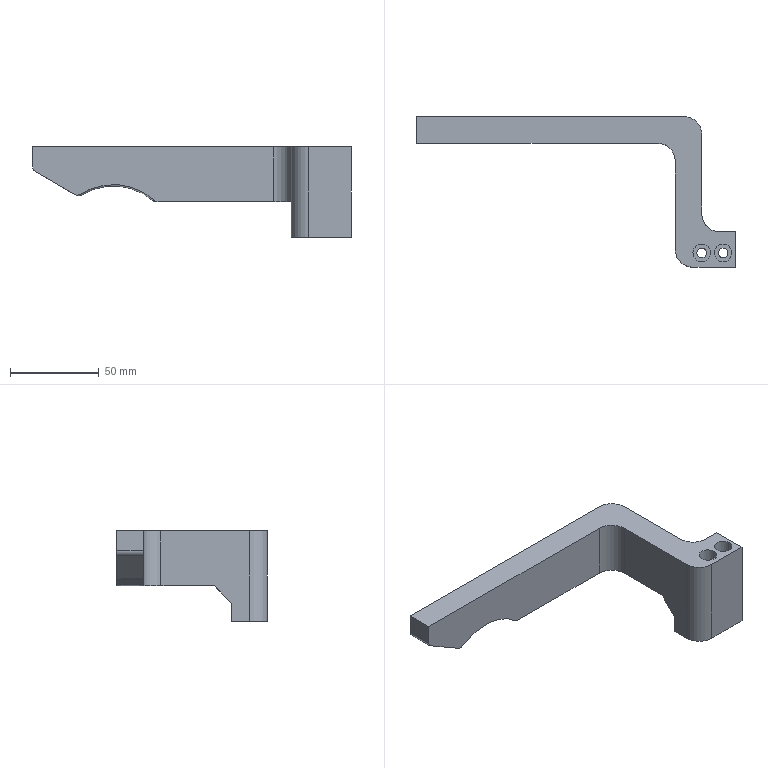NC program | NX | posted with a generic post | part box 180 x 85 x 51 mm
Lines 24 to 1125 of 44959:
(ADAPTIVE_MILLING , TOOL : D12C)
N46 T12 M6
N48 G54
N50 G17 G0 G90 X104.183 Y22.541 S9500 M3
N52 G43 Z30. H12
N54 Z-23.
N56 G94 G1 Z-26. F1000.
N58 X102.633 Y23.218 F3000.
N60 G3 X101.017 Y22.541 R1.217
N62 X100.588 Y19.038 R13.703
N64 X100.502 Y0.139 R864.64
N66 G1 X100.501 Y-45.049
N68 X100.5 Y-45.199
N70 X100.497 Y-45.311
N72 X100.491 Y-45.424
N74 X100.483 Y-45.536
N76 G2 X96.9 Y-50.921 R7.15
N78 X90.805 Y-52.726 R14.272
N80 X81.774 Y-52.986 R105.312
N82 G1 X79.862 Y-52.99
N84 X76.637 Y-52.992
N86 X64.712
N88 X-92.638 Y-52.991
N90 X-92.713 Y-52.99
N92 X-92.826 Y-52.986
N94 G2 X-98.231 Y-49.705 R6.988
N96 X-100.165 Y-43.85 R13.204
N98 X-100.483 Y-34.823 R85.978
N100 G1 X-100.487 Y-33.135
N102 X-100.49 Y-30.548
N104 X-100.491 Y-24.585
N106 Y45.127
N108 X-100.489 Y45.24
N110 X-100.485 Y45.352
N112 G2 X-97.049 Y50.824 R7.048
N114 X-90.979 Y52.706 R13.869
N116 X-81.425 Y52.986 R104.172
N118 G1 X-79.362 Y52.989
N120 X-75.575 Y52.991
N122 X-41.112
N124 X92.65
N126 X92.763 Y52.989
N128 X92.875 Y52.984
N130 G2 X98.336 Y49.53 R7.063
N132 X100.198 Y43.532 R13.787
N134 X100.485 Y34.128 R99.972
N136 X100.443 Y24.191 R284.848
N138 G3 X100.015 Y11.078 R148.084
N140 G1 X100.011 Y8.978
N142 X100.009 Y5.453
N144 X100.008 Y-5.872
N146 X100.007 Y-42.622
N148 Y-42.735
N150 X100.004 Y-42.885
N152 G2 X95.318 Y-50.333 R8.732
N154 X88.759 Y-52.177 R16.71
N156 X79.355 Y-52.477 R105.888
N158 G1 X77.705 Y-52.481
N160 X75.305 Y-52.485
N162 X70.73 Y-52.486
N164 X-31.645
N166 X-33.895 Y-52.49
N168 X-36.108 Y-52.491
N170 X-38.358 Y-52.489
N172 X-40.683 Y-52.491
N174 X-42.858 Y-52.489
N176 X-45.183 Y-52.491
N178 X-47.47 Y-52.489
N180 X-50.245 Y-52.49
N182 X-52.458 Y-52.489
N184 X-54.783 Y-52.49
N186 X-57.07 Y-52.489
N188 X-59.845 Y-52.49
N190 X-62.02 Y-52.489
N192 X-64.345 Y-52.49
N194 X-66.633 Y-52.489
N196 X-69.295 Y-52.49
N198 X-71.583 Y-52.489
N200 X-73.908 Y-52.49
N202 X-76.195 Y-52.489
N204 X-78.97 Y-52.49
N206 X-81.183 Y-52.489
N208 X-83.508 Y-52.49
N210 X-85.795 Y-52.489
N212 X-88.57 Y-52.49
N214 X-90.258 Y-52.489
N216 X-90.408 Y-52.487
N218 X-90.558 Y-52.482
N220 X-90.708 Y-52.476
N222 X-90.82 Y-52.469
N224 G2 X-97.829 Y-47.823 R8.734
N226 X-99.685 Y-41.19 R16.83
N228 X-99.979 Y-30.96 R119.013
N230 G1 X-99.982 Y-28.973
N232 X-99.985 Y-25.673
N234 X-99.986 Y-15.585
N236 X-99.985 Y42.765
N238 X-99.983 Y42.915
N240 X-99.978 Y43.064
N242 G2 X-95.308 Y50.33 R8.727
N244 X-88.749 Y52.175 R16.689
N246 X-77.995 Y52.48 R120.763
N248 G1 X-75.745 Y52.483
N250 X-71.77 Y52.485
N252 X-43.458 Y52.486
N254 X90.267 Y52.485
N256 X90.38 Y52.483
N258 X90.492 Y52.481
N260 G2 X97.756 Y47.936 R8.688
N262 X99.651 Y41.47 R16.28
N264 X99.977 Y31.467 R104.384
N266 X99.663 Y19.737 R156.739
N268 G3 X99.514 Y0.726 R633.906
N270 G1 X99.513 Y-40.261
N272 X99.512 Y-40.524
N274 X99.51 Y-40.749
N276 X99.507 Y-40.974
N278 X99.5 Y-41.198
N280 X99.492 Y-41.386
N282 G2 X93.807 Y-49.9 R9.898
N284 X86.723 Y-51.686 R19.459
N286 X75.967 Y-51.974 R137.207
N288 G1 X73.867 Y-51.978
N290 X70.492 Y-51.98
N292 X61.23 Y-51.981
N294 X-29.22 Y-51.98
N296 X-31.545 Y-51.985
N298 X-33.833 Y-51.986
N300 X-35.97
N302 X-38.295 Y-51.988
N304 X-40.583
N306 X-41.558 Y-51.987
N308 X-43.883 Y-51.989
N310 X-46.17 Y-51.988
N312 X-46.508
N314 X-48.758 Y-51.989
N316 X-50.82 Y-51.987
N318 X-53.07 Y-51.988
N320 X-55.133 Y-51.987
N322 X-57.458 Y-51.988
N324 X-59.745 Y-51.987
N326 X-62.258 Y-51.988
N328 X-64.583 Y-51.987
N330 X-66.833 Y-51.988
N332 X-68.745 Y-51.986
N334 X-70.995 Y-51.988
N336 X-72.908 Y-51.987
N338 X-75.158 Y-51.988
N340 X-77.258 Y-51.987
N342 X-79.508 Y-51.989
N344 X-81.608 Y-51.987
N346 X-83.858 Y-51.989
N348 X-85.958 Y-51.988
N350 G2 X-90.261 Y-51.823 R26.749
N352 X-97.485 Y-46.13 R9.964
N354 X-99.186 Y-39.213 R19.73
N356 X-99.473 Y-28.383 R138.479
N358 G1 X-99.477 Y-26.283
N360 X-99.479 Y-22.87
N362 X-99.48 Y-13.083
N364 Y40.617
N366 X-99.478 Y40.805
N368 X-99.476 Y40.955
N370 G2 X-93.801 Y49.893 R9.889
N372 X-86.83 Y51.673 R19.285
N374 X-76.375 Y51.971 R128.078
N376 G1 X-74.463 Y51.975
N378 X-71.575 Y51.978
N380 X-65.35 Y51.98
N382 X88.1 Y51.979
N384 X88.287 Y51.978
N386 X88.512 Y51.975
N388 G2 X97.385 Y46.316 R9.878
N390 X99.185 Y39.198 R19.477
N392 X99.224 Y21.172 R144.828
N394 G3 X99.013 Y0.362 R556.134
N396 G1 X99.011 Y-1.551
N398 X99.012 Y-3.801
N400 X99.011 Y-5.638
N402 X99.013 Y-7.963
N404 X99.011 Y-10.251
N406 X99.012 Y-11.376
N408 Y-13.663
N410 X99.011 Y-15.276
N412 X99.012 Y-17.601
N414 X99.011 Y-19.888
N416 X99.012 Y-22.438
N418 X99.011 Y-24.238
N420 X99.012 Y-26.563
N422 X99.011 Y-28.851
N424 Y-29.113
N426 X99.012 Y-31.363
N428 X99.01 Y-33.313
N430 G2 X98.946 Y-40.436 R135.893
N432 X92.544 Y-49.421 R10.75
N434 X85.327 Y-51.161 R21.244
N436 X74.46 Y-51.466 R137.759
N438 G1 X72.622 Y-51.47
N440 X69.885 Y-51.473
N442 X64.597 Y-51.475
N444 X4.11
N446 X1.86 Y-51.479
N448 X-0.353 Y-51.48
N450 X-2.603 Y-51.478
N452 X-4.853 Y-51.479
N454 X-6.615 Y-51.478
N456 X-8.865 Y-51.479
N458 X-10.89 Y-51.478
N460 X-13.14 Y-51.479
N462 X-15.165 Y-51.478
N464 X-17.415 Y-51.479
N466 X-19.403 Y-51.478
N468 X-21.653 Y-51.479
N470 X-23.678 Y-51.478
N472 X-25.928 Y-51.479
N474 X-27.39 Y-51.478
N476 X-29.715 Y-51.481
N478 X-30.765
N480 X-33.015 Y-51.485
N482 X-35.228 Y-51.486
N484 X-36.39 Y-51.485
N486 X-38.64 Y-51.487
N488 X-40.853 Y-51.486
N490 X-43.59 Y-51.488
N492 X-45.578 Y-51.486
N494 X-47.828 Y-51.487
N496 X-49.89 Y-51.486
N498 X-52.215 Y-51.487
N500 X-54.503 Y-51.486
N502 X-57.053 Y-51.487
N504 X-58.928 Y-51.486
N506 X-61.253 Y-51.487
N508 X-63.54 Y-51.486
N510 X-66.278
N512 X-67.853 Y-51.485
N514 X-70.103 Y-51.486
N516 X-71.94 Y-51.485
N518 X-74.19 Y-51.487
N520 X-76.253 Y-51.486
N522 X-78.503 Y-51.487
N524 X-80.565 Y-51.486
N526 X-82.815 Y-51.487
N528 X-84.878 Y-51.486
N530 G2 X-89.654 Y-51.157 R20.334
N532 X-96.946 Y-44.982 R10.805
N534 X-98.662 Y-37.797 R21.426
N536 X-98.964 Y-27.042 R137.503
N538 G1 X-98.969 Y-25.167
N540 X-98.972 Y-22.429
N542 X-98.974 Y-17.217
N544 Y38.771
N546 X-98.972 Y39.071
N548 X-98.97 Y39.258
N550 G2 X-92.432 Y49.462 R10.813
N552 X-84.945 Y51.195 R22.037
N554 X-72.838 Y51.469 R170.072
N556 G1 X-70.176 Y51.472
N558 X-65.226 Y51.474
N560 X86.274
N562 X86.574 Y51.472
N564 X86.762 Y51.469
N566 X86.949 Y51.466
N568 G2 X96.9 Y45.064 R10.771
N570 X98.663 Y37.777 R21.258
N572 X98.79 Y23.012 R121.633
N574 G3 X98.51 Y0.365 R561.198
N576 G1 X98.511 Y-1.96
N578 X98.509 Y-3.835
N580 X98.511 Y-6.16
N582 X98.509 Y-8.448
N584 X98.511 Y-10.96
N586 X98.509 Y-13.21
N588 X98.51 Y-15.722
N590 X98.509 Y-18.01
N592 X98.51 Y-20.41
N594 X98.509 Y-22.735
N596 X98.511 Y-25.06
N598 X98.509 Y-27.347
N600 Y-27.647
N602 X98.51 Y-29.972
N604 X98.509 Y-32.297
N606 X98.511 Y-34.622
N608 G2 X98.321 Y-40.126 R39.885
N610 X91.512 Y-48.883 R11.401
N612 X84.141 Y-50.633 R22.526
N614 X73.162 Y-50.958 R136.895
N616 G1 X71.399 Y-50.963
N618 X68.924 Y-50.967
N620 X64.799 Y-50.969
N622 X49.499
N624 X6.524
N626 X4.199 Y-50.974
N628 X1.912 Y-50.975
N630 X-0.263 Y-50.974
N632 X-2.588 Y-50.977
N634 X-4.876
N636 X-5.888 Y-50.976
N638 X-8.213 Y-50.978
N640 X-10.501 Y-50.977
N642 X-10.838
N644 X-13.163 Y-50.978
N646 X-15.451 Y-50.977
N648 X-18.188
N650 X-19.763 Y-50.976
N652 X-22.088 Y-50.978
N654 X-24.376 Y-50.977
N656 X-24.901 Y-50.976
N658 X-27.151 Y-50.977
N660 X-27.863
N662 X-30.113 Y-50.979
N664 X-31.126 Y-50.98
N666 X-33.376 Y-50.984
N668 X-35.588 Y-50.985
N670 X-37.051 Y-50.984
N672 X-39.301 Y-50.986
N674 X-41.513 Y-50.985
N676 X-44.176 Y-50.987
N678 X-46.463 Y-50.985
N680 X-47.176 Y-50.984
N682 X-49.426 Y-50.985
N684 X-50.701 Y-50.984
N686 X-52.951 Y-50.986
N688 X-55.163 Y-50.985
N690 X-55.538 Y-50.984
N692 X-57.788 Y-50.985
N694 X-59.401 Y-50.984
N696 X-61.726 Y-50.986
N698 X-64.013 Y-50.985
N700 X-64.876 Y-50.984
N702 X-67.126
N704 X-68.476 Y-50.983
N706 X-70.726 Y-50.985
N708 X-72.751 Y-50.984
N710 X-75.001 Y-50.985
N712 G2 X-86.437 Y-50.929 R334.978
N714 X-96.37 Y-44.025 R11.416
N716 X-98.16 Y-36.32 R22.954
N718 X-98.461 Y-24.177 R164.437
N720 G1 X-98.465 Y-21.852
N722 X-98.468 Y-18.102
N724 X-98.469 Y-7.415
N726 X-98.468 Y37.135
N728 Y37.285
N730 X-98.465 Y37.623
N732 G2 X-96.76 Y44.366 R12.529
N734 X-89.843 Y49.53 R12.587
N736 X-81.717 Y50.8 R30.53
N738 X-64.395 Y50.968 R454.906
N740 G1 X-44.407
N742 X84.63
N744 X84.78 Y50.967
N746 X85.118 Y50.964
N748 X85.38 Y50.96
N750 X85.68 Y50.952
N752 G2 X94.217 Y47.301 R11.485
N754 X97.644 Y40.029 R15.153
N756 X98.396 Y31.298 R49.905
N758 X98.156 Y18.965 R259.207
N760 G3 X98.009 Y-4.322 R927.895
N762 G1 X98.007 Y-6.459
N764 X98.009 Y-8.784
N766 X98.007 Y-11.034
N768 X98.008 Y-13.547
N770 X98.007 Y-15.872
N772 X98.008 Y-18.197
N774 X98.007 Y-20.522
N776 X98.008 Y-22.847
N778 G2 X97.966 Y-37.321 R804.806
N780 X94.215 Y-45.957 R12.099
N782 X86.962 Y-49.517 R15.409
N784 X78.393 Y-50.366 R46.017
N786 X60.018 Y-50.464 R838.629
N788 G1 X8.943
N790 X6.618 Y-50.468
N792 X4.331 Y-50.47
N794 X1.893
N796 X-0.432 Y-50.474
N798 X-2.719 Y-50.475
N800 X-4.444 Y-50.474
N802 X-6.769 Y-50.476
N804 X-9.057
N806 X-9.694 Y-50.475
N808 X-12.019 Y-50.477
N810 X-14.307 Y-50.475
N812 X-14.682
N814 X-16.932 Y-50.476
N816 X-18.694 Y-50.475
N818 X-21.019 Y-50.477
N820 X-23.307 Y-50.475
N822 X-23.832
N824 X-26.157 Y-50.476
N826 X-27.432 Y-50.475
N828 X-29.757 Y-50.478
N830 X-31.032 Y-50.479
N832 X-33.282 Y-50.482
N834 X-35.494 Y-50.483
N836 X-36.657
N838 X-38.907 Y-50.484
N840 X-41.157
N842 X-43.407 Y-50.485
N844 X-45.619 Y-50.484
N846 X-46.144 Y-50.483
N848 X-48.469 Y-50.484
N850 X-50.269 Y-50.483
N852 X-52.594 Y-50.485
N854 X-54.882 Y-50.484
N856 X-55.519 Y-50.483
N858 X-57.769 Y-50.484
N860 X-59.194 Y-50.483
N862 X-61.444 Y-50.485
N864 X-63.657 Y-50.483
N866 X-64.219
N868 X-66.469
N870 G2 X-84.881 Y-50.441 R991.792
N872 X-91.413 Y-48.478 R12.976
N874 X-95.973 Y-43.934 R6.278
N876 X-97.794 Y-33.025 R38.287
N878 X-97.962 Y-15.252 R491.479
N880 G1 X-97.963 Y0.948
N882 Y35.598
N884 X-97.962 Y35.786
N886 X-97.959 Y36.123
N888 X-97.955 Y36.423
N890 X-97.95 Y36.686
N892 G2 X-95.932 Y43.912 R13.045
N894 X-88.775 Y49.02 R13.286
N896 X-80.795 Y50.269 R31.53
N898 X-63.623 Y50.462 R400.009
N900 G1 X-52.748 Y50.463
N902 X83.077 Y50.462
N904 X83.302
N906 X83.602 Y50.459
N908 X83.902 Y50.455
N910 X84.127 Y50.451
N912 G2 X91.397 Y48.481 R13.562
N914 X95.973 Y43.934 R6.277
N916 X97.776 Y33.361 R37.715
N918 X97.743 Y22.227 R138.477
N920 G3 X97.506 Y-5.183 R921.948
N922 G1 X97.507 Y-7.508
N924 X97.506 Y-9.796
N926 X97.507 Y-12.121
N928 X97.505 Y-14.446
N930 X97.507 Y-16.771
N932 X97.505 Y-19.021
N934 X97.507 Y-21.533
N936 X97.505 Y-23.821
N938 G2 X97.446 Y-36.42 R413.025
N940 X93.853 Y-44.997 R12.689
N942 X86.332 Y-48.909 R15.522
N944 X77.359 Y-49.85 R45.736
N946 X60.935 Y-49.957 R763.704
N948 G1 X45.335 Y-49.958
N950 X11.36
N952 X9.035 Y-49.962
N954 X6.747 Y-49.964
N956 X4.272
N958 X1.947 Y-49.969
N960 X-0.34 Y-49.97
N962 X-2.028
N964 X-4.353 Y-49.973
N966 X-6.64 Y-49.974
N968 X-7.878 Y-49.973
N970 X-10.203 Y-49.975
N972 X-12.49 Y-49.974
N974 X-13.053 Y-49.973
N976 X-15.378 Y-49.975
N978 X-17.665 Y-49.973
N980 X-19.99 Y-49.975
N982 X-22.278 Y-49.974
N984 X-22.803 Y-49.973
N986 X-25.128 Y-49.975
N988 X-26.628 Y-49.974
N990 X-28.878 Y-49.976
N992 X-29.965
N994 X-32.215 Y-49.98
N996 X-34.428
N998 X-34.99
N1000 X-37.24 Y-49.982
N1002 X-39.453 Y-49.981
N1004 X-42.228 Y-49.983
N1006 X-44.515 Y-49.982
N1008 X-45.04
N1010 X-47.365 Y-49.983
N1012 X-49.503 Y-49.982
N1014 X-51.828 Y-49.984
N1016 X-54.115 Y-49.982
N1018 X-54.715
N1020 X-57.04 Y-49.983
N1022 X-58.99 Y-49.982
N1024 X-61.315 Y-49.984
N1026 X-63.603 Y-49.982
N1028 X-64.578 Y-49.981
N1030 X-66.828 Y-49.982
N1032 X-68.14 Y-49.981
N1034 X-70.465 Y-49.982
N1036 X-72.753 Y-49.981
N1038 X-73.09
N1040 X-75.34 Y-49.982
N1042 X-76.878 Y-49.981
N1044 G2 X-84.525 Y-49.88 R113.76
N1046 X-89.461 Y-48.669 R19.083
N1048 X-91.434 Y-48.473 R27.743
N1050 G1 X-91.3 Y-48.504
N1052 X-89.965 Y-48.65
N1054 X-89.614
N1056 G2 X-86.891 Y-49.168 R25.774
N1058 G3 X-79.306 Y-49.667 R43.084
N1060 G1 X-78.368 Y-49.672
N1062 X-76.756 Y-49.676
N1064 X-74.918 Y-49.678
N1066 X-73.793 Y-49.679
N1068 X-73.156 Y-49.68
N1070 X-71.731
N1072 X-70.756 Y-49.681
N1074 X-69.818 Y-49.68
N1076 X-69.368
N1078 X-68.018 Y-49.681
N1080 X-67.306
N1082 X-66.818 Y-49.682
N1084 X-66.443 Y-49.681
N1086 X-65.731 Y-49.682
N1088 X-65.168
N1090 X-63.781 Y-49.683
N1092 X-62.281
N1094 X-61.718
N1096 X-60.931 Y-49.682
N1098 X-60.293
N1100 X-59.206 Y-49.683
N1102 X-58.493
N1104 X-58.043
N1106 X-56.581 Y-49.682
N1108 X-54.743 Y-49.683
N1110 X-53.431
N1112 X-52.906
N1114 X-52.456
N1116 X-50.993 Y-49.682
N1118 X-50.506 Y-49.683
N1120 X-49.831
N1122 X-49.418
N1124 X-48.518
N1126 X-46.681 Y-49.682
N1128 X-45.968 Y-49.683
N1130 X-44.693
N1132 X-44.131
N1134 X-43.043
N1136 X-42.518
N1138 X-41.393 Y-49.682
N1140 X-40.868
N1142 X-39.893 Y-49.683
N1144 X-39.556 Y-49.682
N1146 X-39.181 Y-49.683
N1148 X-38.168 Y-49.682
N1150 X-37.643
N1152 X-37.118 Y-49.681
N1154 X-36.706
N1156 X-34.943
N1158 X-34.606
N1160 X-34.268
N1162 X-33.556 Y-49.68
N1164 X-32.806
N1166 X-31.681 Y-49.678
N1168 X-31.231
N1170 X-30.331 Y-49.677
N1172 X-29.993
N1174 X-28.193 Y-49.675
N1176 X-27.706
N1178 X-26.356
N1180 X-25.793
N1182 X-24.218 Y-49.674
N1184 X-23.768
N1186 X-23.168 Y-49.675
N1188 X-22.718 Y-49.674
N1190 X-22.118
N1192 X-20.993 Y-49.675
N1194 X-20.281
N1196 X-18.931 Y-49.674
N1198 X-18.443
N1200 X-18.106
N1202 X-17.656
N1204 X-16.981 Y-49.675
N1206 X-15.931 Y-49.674
N1208 X-15.518 Y-49.675
N1210 X-14.468 Y-49.674
N1212 X-13.343 Y-49.675
N1214 X-12.856
N1216 X-11.768
N1218 X-10.343 Y-49.674
N1220 X-9.181 Y-49.673
N1222 X-8.056 Y-49.674
N1224 X-7.343
N1226 X-5.506 Y-49.673
N1228 X-3.968 Y-49.671
N1230 X-2.243
N1232 X-1.156
N1234 X-0.106 Y-49.67
N1236 X0.419 Y-49.669
N1238 X0.982
N1240 X1.732 Y-49.668
N1242 X2.632 Y-49.666
N1244 X4.919
N1246 X6.007 Y-49.665
N1248 X7.619 Y-49.663
N1250 X7.994
N1252 X8.782 Y-49.662
N1254 X9.457 Y-49.66
N1256 X10.282
N1258 X11.782 Y-49.659
N1260 X13.132
N1262 X13.469 Y-49.658
N1264 X13.882 Y-49.659
N1266 X14.482 Y-49.658
N1268 X14.932
N1270 X15.607
N1272 X16.732
N1274 X17.332
N1276 X17.969
N1278 X18.719
N1280 X19.469
N1282 X20.219
N1284 X21.082
N1286 X21.569
N1288 X22.019
N1290 X23.369
N1292 X24.494
N1294 X25.057
N1296 X25.769
N1298 X26.144
N1300 X27.119
N1302 X28.507
N1304 X30.269 Y-49.657
N1306 X30.644 Y-49.658
N1308 X31.057 Y-49.657
N1310 X32.444 Y-49.658
N1312 X32.969 Y-49.657
N1314 X33.307 Y-49.658
N1316 X33.719 Y-49.657
N1318 X35.069 Y-49.658
N1320 X35.594
N1322 X36.007
N1324 X36.344
N1326 X36.719
N1328 X37.694
N1330 X39.082
N1332 X40.844
N1334 X41.182
N1336 X41.594
N1338 X42.194 Y-49.657
N1340 X42.682 Y-49.658
N1342 X43.882 Y-49.657
N1344 X45.007
N1346 X45.569 Y-49.658
N1348 X46.432
N1350 X46.844
N1352 X47.819
N1354 X48.757
N1356 X49.732
N1358 X50.669
N1360 X51.644
N1362 X53.032
N1364 X53.632
N1366 X54.869 Y-49.657
N1368 X55.207 Y-49.658
N1370 X56.332 Y-49.657
N1372 X56.669 Y-49.658
N1374 X57.119 Y-49.657
N1376 X58.282
N1378 X58.844 Y-49.658
N1380 X59.519
N1382 X59.932 Y-49.657
N1384 X61.057
N1386 X61.582
N1388 X63.157 Y-49.656
N1390 X63.494
N1392 X64.207 Y-49.655
N1394 X65.032 Y-49.654
N1396 X65.482
N1398 G3 X80.028 Y-49.412 R272.344
N1400 X88.228 Y-47.93 R29.327
N1402 X95.619 Y-41.556 R12.873
N1404 X97.103 Y-34.791 R17.08
N1406 X97.206 Y-19.267 R485.423
N1408 G1 Y-17.28
N1410 X97.205 Y-16.005
N1412 X97.206 Y-15.217
N1414 Y-13.38
N1416 Y-12.855
N1418 Y-12.217
N1420 Y-11.092
N1422 X97.207 Y-8.805
N1424 X97.206 Y-6.967
N1426 X97.207 Y-6.217
N1428 X97.208 Y-4.68
N1430 Y-3.517
N1432 Y-2.242
N1434 G2 X97.564 Y27.679 R972.698
N1436 G3 X96.866 Y38.93 R64.756
N1438 X96.15 Y42.203 R153.829
N1440 X95.973 Y43.934 R27.64
N1442 G1 X96.004 Y43.8
N1444 X96.15 Y42.465
N1446 Y42.203
N1448 G3 X96.568 Y37.613 R40.294
N1450 G2 X96.967 Y23.642 R101.585
N1452 G3 X96.705 Y-4.968 R948.71
N1454 G1 X96.706 Y-7.293
N1456 X96.704 Y-9.393
N1458 X96.705 Y-11.718
N1460 X96.703 Y-14.005
N1462 X96.705 Y-16.518
N1464 X96.703 Y-18.805
N1466 Y-19.068
N1468 X96.704 Y-21.393
N1470 X96.702 Y-23.68
N1472 G2 X96.553 Y-34.74 R197.136
N1474 X94.464 Y-41.901 R15.206
N1476 X87.041 Y-47.503 R13.787
N1478 X78.935 Y-48.899 R31.253
N1480 X63.676 Y-49.154 R291.014
N1482 G1 X63.076 Y-49.156
N1484 X60.826 Y-49.158
N1486 X58.276 Y-49.159
N1488 X56.851 Y-49.16
N1490 X54.601 Y-49.159
N1492 X52.726 Y-49.16
N1494 X50.476 Y-49.159
N1496 X48.676 Y-49.16
N1498 X46.426 Y-49.159
N1500 X44.214 Y-49.16
N1502 X41.964 Y-49.159
N1504 X40.014 Y-49.16
N1506 X37.764 Y-49.159
N1508 X35.589 Y-49.16
N1510 X33.339 Y-49.159
N1512 X31.464 Y-49.16
N1514 X29.214 Y-49.159
N1516 X27.001 Y-49.161
N1518 X24.564 Y-49.16
N1520 X22.764 Y-49.161
N1522 X20.514 Y-49.16
N1524 X18.714 Y-49.161
N1526 X16.464 Y-49.159
N1528 X14.251 Y-49.161
N1530 X13.801
N1532 X11.551
N1534 X9.339 Y-49.163
N1536 X8.139 Y-49.165
N1538 X5.889 Y-49.167
N1540 X4.951 Y-49.168
N1542 X2.701
N1544 X0.489 Y-49.17
N1546 X0.001 Y-49.171
N1548 X-2.249 Y-49.172
N1550 X-3.824 Y-49.174
N1552 X-6.074
N1554 X-7.274 Y-49.176
N1556 X-9.524 Y-49.175
N1558 X-11.624 Y-49.176
N1560 X-13.874
N1562 X-15.561 Y-49.177
N1564 X-17.811 Y-49.176
N1566 X-19.949 Y-49.177
N1568 X-22.199 Y-49.176
N1570 X-24.411 Y-49.178
N1572 X-26.661 Y-49.177
N1574 X-28.874 Y-49.179
N1576 X-29.361
N1578 X-31.611
N1580 X-33.711 Y-49.182
N1582 X-35.961
N1584 X-37.724 Y-49.184
N1586 X-39.974
N1588 X-41.399 Y-49.185
N1590 X-43.649 Y-49.184
N1592 X-45.524 Y-49.186
N1594 X-47.774 Y-49.184
N1596 X-49.986 Y-49.186
N1598 X-52.236 Y-49.185
N1600 X-53.699
N1602 X-55.949 Y-49.183
N1604 X-58.161 Y-49.185
N1606 X-58.424
N1608 X-60.674 Y-49.183
N1610 X-62.886 Y-49.185
N1612 X-65.136 Y-49.184
N1614 G2 X-82.122 Y-49.09 R597.144
N1616 X-86.378 Y-48.65 R40.76
N1618 G1 X-89.528
N1620 X-86.378
N1622 G2 X-79.106 Y-48.849 R894.652
N1624 G1 X-78.319 Y-48.858
N1626 X-77.344 Y-48.865
N1628 X-75.956 Y-48.871
N1630 X-74.269 Y-48.876
N1632 X-72.919 Y-48.878
N1634 X-71.906 Y-48.879
N1636 X-70.894
N1638 X-69.919 Y-48.88
N1640 X-68.756 Y-48.881
N1642 X-68.006 Y-48.882
N1644 X-67.331
N1646 X-66.544
N1648 X-65.869 Y-48.883
N1650 X-65.456
N1652 X-64.931 Y-48.884
N1654 X-63.694 Y-48.883
N1656 X-62.869
N1658 X-62.531
N1660 X-62.081
N1662 X-61.369
N1664 X-60.881 Y-48.884
N1666 X-58.669 Y-48.883
N1668 X-58.256 Y-48.884
N1670 X-57.919 Y-48.883
N1672 X-57.506 Y-48.884
N1674 X-56.194
N1676 X-55.669
N1678 X-54.581
N1680 X-54.131
N1682 X-53.231
N1684 X-52.819
N1686 X-52.444 Y-48.885
N1688 X-51.694
N1690 X-50.981
N1692 X-50.494
N1694 X-50.119
N1696 X-49.781 Y-48.884
N1698 X-48.656 Y-48.885
N1700 X-48.131
N1702 X-47.344
N1704 X-46.856
N1706 X-46.331
N1708 X-45.806
N1710 X-45.394
N1712 X-44.494
N1714 X-44.044 Y-48.884
N1716 X-42.956 Y-48.885
N1718 X-41.831 Y-48.884
N1720 X-40.819
N1722 X-39.806
N1724 X-39.431
N1726 X-38.981
N1728 X-37.856 Y-48.883
N1730 X-35.981 Y-48.882
N1732 X-35.119
N1734 X-34.331 Y-48.881
N1736 X-33.769
N1738 X-32.756
N1740 X-31.256 Y-48.88
N1742 X-30.431 Y-48.879
N1744 X-29.456 Y-48.878
N1746 X-28.219 Y-48.877
N1748 X-26.269 Y-48.878
N1750 X-25.594
N1752 X-25.219 Y-48.877
N1754 X-24.506
N1756 X-23.456
N1758 X-22.931
N1760 X-21.356
N1762 X-20.681
N1764 X-20.231 Y-48.876
N1766 X-19.031
N1768 X-18.319
N1770 X-17.156 Y-48.877
N1772 X-16.106 Y-48.876
N1774 X-15.244
N1776 X-14.831 Y-48.875
N1778 X-13.106 Y-48.876
N1780 X-12.619
N1782 X-12.094
N1784 X-11.494
N1786 X-10.481 Y-48.875
N1788 X-10.031
N1790 X-8.756 Y-48.876
N1792 X-8.344 Y-48.875
N1794 X-7.969
N1796 X-7.594
N1798 X-6.694
N1800 X-6.319 Y-48.874
N1802 X-5.831 Y-48.875
N1804 X-5.081 Y-48.874
N1806 X-4.219 Y-48.873
N1808 X-3.881
N1810 X-3.469
N1812 X-3.131
N1814 X-2.606 Y-48.872
N1816 X-2.119
N1818 X-1.706
N1820 X-0.994 Y-48.871
N1822 X-0.356 Y-48.87
N1824 X0.656
N1826 X0.994 Y-48.869
N1828 X1.444
N1830 X2.869
N1832 X3.994 Y-48.868
N1834 X4.969 Y-48.867
N1836 X5.344
N1838 X6.356 Y-48.866
N1840 X7.219 Y-48.865
N1842 X8.044 Y-48.864
N1844 X8.869 Y-48.863
N1846 X9.431 Y-48.862
N1848 X9.881
N1850 X11.231
N1852 X11.981
N1854 X12.506
N1856 X12.994 Y-48.861
N1858 X13.594
N1860 X13.969 Y-48.86
N1862 X15.056
N1864 X15.581
N1866 X17.344 Y-48.861
N1868 X17.681
N1870 X18.056
N1872 X18.656
N1874 X19.294
N1876 X20.044
N1878 X21.056
N1880 X21.619 Y-48.86
N1882 X22.294
N1884 X22.706
N1886 X23.944
N1888 X24.431
N1890 X25.406 Y-48.861
N1892 X25.969 Y-48.86
N1894 X27.956
N1896 X29.531
N1898 X30.919
N1900 X31.294
N1902 X32.306 Y-48.859
N1904 X33.994 Y-48.86
N1906 X34.706
N1908 X35.156
N1910 X36.056
N1912 X36.694
N1914 X37.444
N1916 X38.981
N1918 X39.469
N1920 X39.806
N1922 X40.219 Y-48.859
N1924 X40.556 Y-48.86
N1926 X41.081
N1928 X41.569 Y-48.859
N1930 X42.581 Y-48.86
N1932 X43.069
N1934 X43.594 Y-48.859
N1936 X44.719 Y-48.86
N1938 X45.506
N1940 X46.256
N1942 X47.269
N1944 X48.244 Y-48.859
N1946 X48.656 Y-48.86
N1948 X49.669 Y-48.859
N1950 X51.469 Y-48.86
N1952 X52.406 Y-48.859
N1954 X53.381 Y-48.86
N1956 X53.906
N1958 X54.619
N1960 X56.156
N1962 X56.531 Y-48.859
N1964 X56.906
N1966 X58.069
N1968 X58.819
N1970 X59.531 Y-48.858
N1972 X61.406 Y-48.857
N1974 G3 X77.828 Y-48.643 R386.619
N1976 X86.361 Y-47.303 R33.413
N1978 X93.964 Y-41.651 R13.696
N1980 X96.16 Y-34.436 R16.254
N1982 X96.392 Y-26.755 R93.343
N1984 G1 X96.399 Y-23.342
N1986 X96.403 Y-19.367
N1988 X96.405 Y-15.392
N1990 X96.404 Y-11.417
N1992 X96.403 Y-10.555
N1994 X96.404 Y-10.18
N1996 X96.405 Y-9.13
N1998 Y-7.48
N2000 X96.404 Y-6.242
N2002 X96.406 Y-5.267
N2004 Y-4.892
N2006 Y-4.517
N2008 Y-3.43
N2010 Y-2.905
N2012 X96.407 Y-2.342
N2014 X96.409 Y-0.092
N2016 Y0.283
N2018 X96.41 Y1.183
N2020 X96.412 Y2.608
N2022 Y2.945
N2024 X96.426 Y7.745
N2026 X96.431 Y8.645
N2028 G2 X96.717 Y26.755 R943.086
N2030 G3 X96.15 Y38.508 R91.827
N2032 G1 Y41.658
N2034 Y31.271
N2036 X96.153 Y31.158
N2038 X96.171 Y30.484
N2040 X96.177 Y30.184
N2042 X96.186 Y29.621
N2044 X96.191 Y29.171
N2046 X96.195 Y28.534
N2048 X96.196 Y27.821
N2050 X96.194 Y27.109
N2052 X96.19 Y26.396
N2054 X96.182 Y25.646
N2056 X96.169 Y24.746
N2058 X96.15 Y23.624
N2060 Y22.535
N2062 X96.13 Y21.747
N2064 X96.099 Y20.473
N2066 X96.064 Y18.861
N2068 X96.04 Y17.623
N2070 X96.019 Y16.498
N2072 X95.998 Y15.149
N2074 X95.982 Y13.986
N2076 X95.968 Y12.824
N2078 X95.952 Y11.286
N2080 X95.94 Y9.861
N2082 X95.932 Y8.587
N2084 X95.923 Y6.637
N2086 X95.915 Y4.312
N2088 X95.913 Y3.187
N2090 X95.909 Y1.537
N2092 X95.907 Y-0.713
N2094 X95.906 Y-1.501
N2096 Y-3.826
N2098 X95.903 Y-5.738
N2100 X95.904 Y-8.063
N2102 X95.902 Y-9.976
N2104 X95.903 Y-12.301
N2106 X95.902 Y-14.288
N2108 X95.903 Y-16.538
N2110 X95.902 Y-18.751
N2112 X95.899 Y-20.213
N2114 Y-22.463
N2116 X95.895 Y-24.676
N2118 G2 X95.613 Y-34.117 R96.602
N2120 X93.025 Y-41.539 R15.384
N2122 X85.312 Y-46.832 R14.543
N2124 X76.733 Y-48.134 R35.249
N2126 X63.904 Y-48.36 R363.77
N2128 G1 X63.573 Y-48.44
N2130 X63.478 Y-48.455
N2132 X61.024 Y-48.648
N2134 X60.976 Y-48.65
N2136 X-85.537
N2138 G3 X-86.361 Y-50.722 R1.201
N2140 X-85.729 Y-51.058 Z-25.97 R1.682
N2142 G1 X-84.156 Y-51.642 Z-25.9
N2144 X-81.997 Y-52.435
N2146 X-81.718 Y-52.468
N2148 X61.204 Y-53.037
N2150 G3 X62.38 Y-52.099 R1.208
N2152 G1 X62.499 Y-51.568
N2154 X63.023 Y-49.226 Z-26.
N2156 G2 X63.904 Y-48.36 R1.213
N2158 X67.86 Y-48.054 R21.123
N2160 G3 X79.473 Y-47.596 R142.714
N2162 X87.556 Y-45.486 R23.473
N2164 X94.879 Y-35.83 R13.61
N2166 X95.552 Y-28.373 R38.708
N2168 X95.602 Y-10.298 R959.404
N2170 G1 X95.603 Y-9.21
N2172 Y-8.235
N2174 Y-7.073
N2176 Y-6.623
N2178 Y-6.285
N2180 X95.604 Y-5.873
N2182 X95.605 Y-4.973
N2184 Y-4.598
N2186 Y-3.51
N2188 X95.606 Y-2.723
N2190 X95.607 Y-1.71
N2192 Y-1.298
N2194 X95.608 Y0.09
N2196 X95.61 Y1.402
N2198 X95.611 Y1.777
N2200 X95.612 Y2.677
N2202 X95.615 Y3.465
N2204 X95.622 Y5.752
N2206 G2 X95.83 Y20.636 R634.202
N2208 G3 X96.15 Y22.535 R7.003
N2210 G1 X96.004 Y21.2
N2212 X95.849 Y20.711
N2214 G3 X95.332 Y17.198 R13.218
N2216 X95.114 Y-0.311 R428.776
N2218 G1 X95.107 Y-2.561
N2220 X95.104 Y-4.774
N2222 X95.103 Y-6.986
N2224 X95.104 Y-8.561
N2226 X95.103 Y-10.811
N2228 X95.104 Y-12.311
N2230 X95.102 Y-14.561
N2232 X95.103 Y-16.699
N2234 G2 X94.945 Y-30.646 R314.796
N2236 X93.427 Y-38.103 R21.684
N2238 X85.196 Y-45.631 R14.017
N2240 X76.751 Y-47.236 R30.366
N2242 X66.709 Y-47.613 R431.695